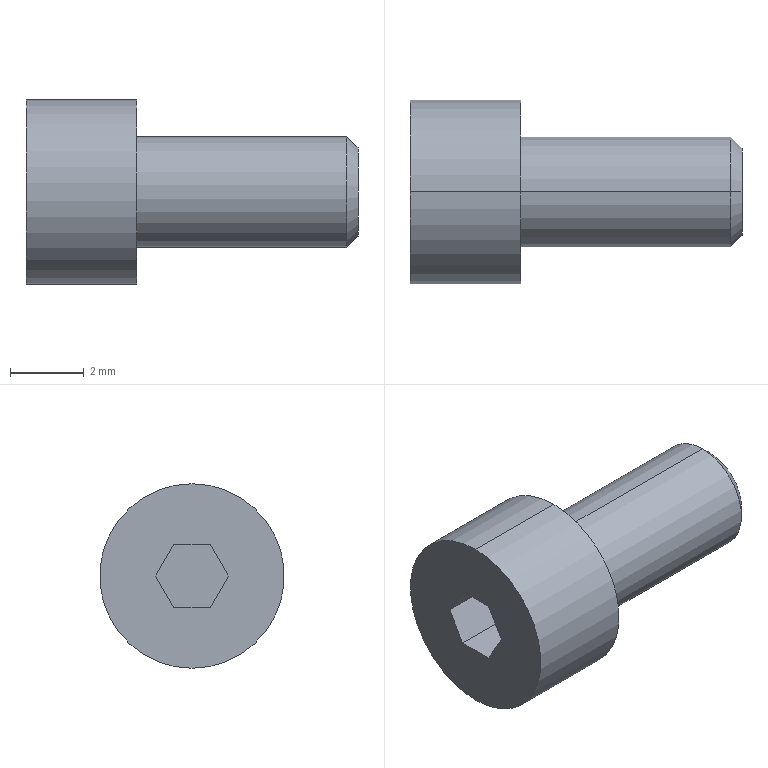Part | SolidWorks | features BaseBody 1 | 1 solid | 16 faces | box 9 x 5 x 5 mm | volume 97.086 mm3 | plane 10 | cylinder 4 | cone 2 | commonest cylinder face diameters 3 x2 5 x2
STEP:
#1=CARTESIAN_POINT('',(9.,0.,1.194));
#2=VERTEX_POINT('',#1);
#3=CARTESIAN_POINT('',(9.,0.,-1.194));
#4=VERTEX_POINT('',#3);
#5=CARTESIAN_POINT('',(9.,0.,0.));
#6=DIRECTION('',(-1.,0.,0.));
#7=DIRECTION('',(0.,0.,1.));
#8=AXIS2_PLACEMENT_3D('',#5,#6,#7);
#9=CIRCLE('',#8,1.194);
#10=EDGE_CURVE('',#2,#4,#9,.T.);
#11=ORIENTED_EDGE('',*,*,#10,.T.);
#12=CARTESIAN_POINT('',(8.694,0.,-1.5));
#13=VERTEX_POINT('',#12);
#14=CARTESIAN_POINT('',(9.,0.,-1.194));
#15=DIRECTION('',(-0.7071,0.,-0.7071));
#16=VECTOR('',#15,1000.);
#17=LINE('',#14,#16);
#18=EDGE_CURVE('',#4,#13,#17,.T.);
#19=ORIENTED_EDGE('',*,*,#18,.T.);
#20=CARTESIAN_POINT('',(8.694,0.,1.5));
#21=VERTEX_POINT('',#20);
#22=CARTESIAN_POINT('',(8.694,0.,0.));
#23=DIRECTION('',(-1.,0.,0.));
#24=DIRECTION('',(0.,0.,1.));
#25=AXIS2_PLACEMENT_3D('',#22,#23,#24);
#26=CIRCLE('',#25,1.5);
#27=EDGE_CURVE('',#21,#13,#26,.T.);
#28=ORIENTED_EDGE('',*,*,#27,.F.);
#29=CARTESIAN_POINT('',(9.,0.,1.194));
#30=DIRECTION('',(-0.7071,0.,0.7071));
#31=VECTOR('',#30,1000.);
#32=LINE('',#29,#31);
#33=EDGE_CURVE('',#2,#21,#32,.T.);
#34=ORIENTED_EDGE('',*,*,#33,.F.);
#35=EDGE_LOOP('',(#11,#19,#28,#34));
#36=FACE_OUTER_BOUND('',#35,.T.);
#37=CARTESIAN_POINT('',(9.,0.,0.));
#38=DIRECTION('',(-1.,0.,0.));
#39=DIRECTION('',(0.,0.,1.));
#40=AXIS2_PLACEMENT_3D('',#37,#38,#39);
#41=CONICAL_SURFACE('',#40,1.194,0.7854);
#42=ADVANCED_FACE('',(#36),#41,.T.);
#43=CARTESIAN_POINT('',(0.,0.,-2.5));
#44=VERTEX_POINT('',#43);
#45=CARTESIAN_POINT('',(0.,0.,2.5));
#46=VERTEX_POINT('',#45);
#47=CARTESIAN_POINT('',(0.,0.,0.));
#48=DIRECTION('',(-1.,0.,0.));
#49=DIRECTION('',(0.,0.,1.));
#50=AXIS2_PLACEMENT_3D('',#47,#48,#49);
#51=CIRCLE('',#50,2.5);
#52=EDGE_CURVE('',#44,#46,#51,.T.);
#53=ORIENTED_EDGE('',*,*,#52,.F.);
#54=CARTESIAN_POINT('',(3.,0.,-2.5));
#55=VERTEX_POINT('',#54);
#56=CARTESIAN_POINT('',(0.,0.,-2.5));
#57=DIRECTION('',(1.,0.,0.));
#58=VECTOR('',#57,1000.);
#59=LINE('',#56,#58);
#60=EDGE_CURVE('',#44,#55,#59,.T.);
#61=ORIENTED_EDGE('',*,*,#60,.T.);
#62=CARTESIAN_POINT('',(3.,0.,2.5));
#63=VERTEX_POINT('',#62);
#64=CARTESIAN_POINT('',(3.,0.,0.));
#65=DIRECTION('',(-1.,0.,0.));
#66=DIRECTION('',(0.,0.,1.));
#67=AXIS2_PLACEMENT_3D('',#64,#65,#66);
#68=CIRCLE('',#67,2.5);
#69=EDGE_CURVE('',#55,#63,#68,.T.);
#70=ORIENTED_EDGE('',*,*,#69,.T.);
#71=CARTESIAN_POINT('',(0.,0.,2.5));
#72=DIRECTION('',(1.,0.,0.));
#73=VECTOR('',#72,1000.);
#74=LINE('',#71,#73);
#75=EDGE_CURVE('',#46,#63,#74,.T.);
#76=ORIENTED_EDGE('',*,*,#75,.F.);
#77=EDGE_LOOP('',(#53,#61,#70,#76));
#78=FACE_OUTER_BOUND('',#77,.T.);
#79=CARTESIAN_POINT('',(0.,0.,0.));
#80=DIRECTION('',(1.,0.,0.));
#81=DIRECTION('',(0.,0.,1.));
#82=AXIS2_PLACEMENT_3D('',#79,#80,#81);
#83=CYLINDRICAL_SURFACE('',#82,2.5);
#84=ADVANCED_FACE('',(#78),#83,.T.);
#85=CARTESIAN_POINT('',(3.,0.,-1.5));
#86=VERTEX_POINT('',#85);
#87=CARTESIAN_POINT('',(3.,0.,1.5));
#88=VERTEX_POINT('',#87);
#89=CARTESIAN_POINT('',(3.,0.,0.));
#90=DIRECTION('',(-1.,0.,0.));
#91=DIRECTION('',(0.,0.,1.));
#92=AXIS2_PLACEMENT_3D('',#89,#90,#91);
#93=CIRCLE('',#92,1.5);
#94=EDGE_CURVE('',#86,#88,#93,.T.);
#95=ORIENTED_EDGE('',*,*,#94,.F.);
#96=CARTESIAN_POINT('',(0.,0.,-1.5));
#97=DIRECTION('',(1.,0.,0.));
#98=VECTOR('',#97,1000.);
#99=LINE('',#96,#98);
#100=EDGE_CURVE('',#86,#13,#99,.T.);
#101=ORIENTED_EDGE('',*,*,#100,.T.);
#102=CARTESIAN_POINT('',(8.694,0.,0.));
#103=DIRECTION('',(-1.,0.,0.));
#104=DIRECTION('',(0.,0.,1.));
#105=AXIS2_PLACEMENT_3D('',#102,#103,#104);
#106=CIRCLE('',#105,1.5);
#107=EDGE_CURVE('',#13,#21,#106,.T.);
#108=ORIENTED_EDGE('',*,*,#107,.T.);
#109=CARTESIAN_POINT('',(0.,0.,1.5));
#110=DIRECTION('',(1.,0.,0.));
#111=VECTOR('',#110,1000.);
#112=LINE('',#109,#111);
#113=EDGE_CURVE('',#88,#21,#112,.T.);
#114=ORIENTED_EDGE('',*,*,#113,.F.);
#115=EDGE_LOOP('',(#95,#101,#108,#114));
#116=FACE_OUTER_BOUND('',#115,.T.);
#117=CARTESIAN_POINT('',(0.,0.,0.));
#118=DIRECTION('',(1.,0.,0.));
#119=DIRECTION('',(0.,0.,1.));
#120=AXIS2_PLACEMENT_3D('',#117,#118,#119);
#121=CYLINDRICAL_SURFACE('',#120,1.5);
#122=ADVANCED_FACE('',(#116),#121,.T.);
#123=CARTESIAN_POINT('',(1.5,0.4949,0.8571));
#124=VERTEX_POINT('',#123);
#125=CARTESIAN_POINT('',(1.5,-0.4949,0.8571));
#126=VERTEX_POINT('',#125);
#127=CARTESIAN_POINT('',(1.5,0.4949,0.8571));
#128=DIRECTION('',(0.,-1.,0.));
#129=VECTOR('',#128,1000.);
#130=LINE('',#127,#129);
#131=EDGE_CURVE('',#124,#126,#130,.T.);
#132=ORIENTED_EDGE('',*,*,#131,.F.);
#133=CARTESIAN_POINT('',(1.5,0.9897,0.));
#134=VERTEX_POINT('',#133);
#135=CARTESIAN_POINT('',(1.5,0.9897,0.));
#136=DIRECTION('',(0.,-0.5,0.866));
#137=VECTOR('',#136,1000.);
#138=LINE('',#135,#137);
#139=EDGE_CURVE('',#134,#124,#138,.T.);
#140=ORIENTED_EDGE('',*,*,#139,.F.);
#141=CARTESIAN_POINT('',(1.5,0.4949,-0.8571));
#142=VERTEX_POINT('',#141);
#143=CARTESIAN_POINT('',(1.5,0.4949,-0.8571));
#144=DIRECTION('',(0.,0.5,0.866));
#145=VECTOR('',#144,1000.);
#146=LINE('',#143,#145);
#147=EDGE_CURVE('',#142,#134,#146,.T.);
#148=ORIENTED_EDGE('',*,*,#147,.F.);
#149=CARTESIAN_POINT('',(1.5,-0.4949,-0.8571));
#150=VERTEX_POINT('',#149);
#151=CARTESIAN_POINT('',(1.5,-0.4949,-0.8571));
#152=DIRECTION('',(0.,1.,0.));
#153=VECTOR('',#152,1000.);
#154=LINE('',#151,#153);
#155=EDGE_CURVE('',#150,#142,#154,.T.);
#156=ORIENTED_EDGE('',*,*,#155,.F.);
#157=CARTESIAN_POINT('',(1.5,-0.9897,0.));
#158=VERTEX_POINT('',#157);
#159=CARTESIAN_POINT('',(1.5,-0.9897,0.));
#160=DIRECTION('',(0.,0.5,-0.866));
#161=VECTOR('',#160,1000.);
#162=LINE('',#159,#161);
#163=EDGE_CURVE('',#158,#150,#162,.T.);
#164=ORIENTED_EDGE('',*,*,#163,.F.);
#165=CARTESIAN_POINT('',(1.5,-0.4949,0.8571));
#166=DIRECTION('',(0.,-0.5,-0.866));
#167=VECTOR('',#166,1000.);
#168=LINE('',#165,#167);
#169=EDGE_CURVE('',#126,#158,#168,.T.);
#170=ORIENTED_EDGE('',*,*,#169,.F.);
#171=EDGE_LOOP('',(#132,#140,#148,#156,#164,#170));
#172=FACE_OUTER_BOUND('',#171,.T.);
#173=CARTESIAN_POINT('',(1.5,0.,0.));
#174=DIRECTION('',(1.,0.,0.));
#175=DIRECTION('',(0.,1.,0.));
#176=AXIS2_PLACEMENT_3D('',#173,#174,#175);
#177=PLANE('',#176);
#178=ADVANCED_FACE('',(#172),#177,.F.);
#179=CARTESIAN_POINT('',(0.,0.9897,0.));
#180=VERTEX_POINT('',#179);
#181=CARTESIAN_POINT('',(0.,0.4949,0.8571));
#182=VERTEX_POINT('',#181);
#183=CARTESIAN_POINT('',(0.,0.9897,0.));
#184=DIRECTION('',(0.,-0.5,0.866));
#185=VECTOR('',#184,1000.);
#186=LINE('',#183,#185);
#187=EDGE_CURVE('',#180,#182,#186,.T.);
#188=ORIENTED_EDGE('',*,*,#187,.F.);
#189=CARTESIAN_POINT('',(1.5,0.9897,0.));
#190=DIRECTION('',(-1.,0.,0.));
#191=VECTOR('',#190,1000.);
#192=LINE('',#189,#191);
#193=EDGE_CURVE('',#134,#180,#192,.T.);
#194=ORIENTED_EDGE('',*,*,#193,.F.);
#195=ORIENTED_EDGE('',*,*,#139,.T.);
#196=CARTESIAN_POINT('',(1.5,0.4949,0.8571));
#197=DIRECTION('',(-1.,0.,0.));
#198=VECTOR('',#197,1000.);
#199=LINE('',#196,#198);
#200=EDGE_CURVE('',#124,#182,#199,.T.);
#201=ORIENTED_EDGE('',*,*,#200,.T.);
#202=EDGE_LOOP('',(#188,#194,#195,#201));
#203=FACE_OUTER_BOUND('',#202,.T.);
#204=CARTESIAN_POINT('',(1.5,0.9897,0.));
#205=DIRECTION('',(0.,-0.866,-0.5));
#206=DIRECTION('',(0.,0.5,-0.866));
#207=AXIS2_PLACEMENT_3D('',#204,#205,#206);
#208=PLANE('',#207);
#209=ADVANCED_FACE('',(#203),#208,.T.);
#210=CARTESIAN_POINT('',(0.,0.4949,-0.8571));
#211=VERTEX_POINT('',#210);
#212=CARTESIAN_POINT('',(0.,0.4949,-0.8571));
#213=DIRECTION('',(0.,0.5,0.866));
#214=VECTOR('',#213,1000.);
#215=LINE('',#212,#214);
#216=EDGE_CURVE('',#211,#180,#215,.T.);
#217=ORIENTED_EDGE('',*,*,#216,.F.);
#218=CARTESIAN_POINT('',(1.5,0.4949,-0.8571));
#219=DIRECTION('',(-1.,0.,0.));
#220=VECTOR('',#219,1000.);
#221=LINE('',#218,#220);
#222=EDGE_CURVE('',#142,#211,#221,.T.);
#223=ORIENTED_EDGE('',*,*,#222,.F.);
#224=ORIENTED_EDGE('',*,*,#147,.T.);
#225=ORIENTED_EDGE('',*,*,#193,.T.);
#226=EDGE_LOOP('',(#217,#223,#224,#225));
#227=FACE_OUTER_BOUND('',#226,.T.);
#228=CARTESIAN_POINT('',(1.5,0.4949,-0.8571));
#229=DIRECTION('',(0.,-0.866,0.5));
#230=DIRECTION('',(-1.,0.,0.));
#231=AXIS2_PLACEMENT_3D('',#228,#229,#230);
#232=PLANE('',#231);
#233=ADVANCED_FACE('',(#227),#232,.T.);
#234=CARTESIAN_POINT('',(0.,-0.4949,-0.8571));
#235=VERTEX_POINT('',#234);
#236=CARTESIAN_POINT('',(0.,-0.4949,-0.8571));
#237=DIRECTION('',(0.,1.,0.));
#238=VECTOR('',#237,1000.);
#239=LINE('',#236,#238);
#240=EDGE_CURVE('',#235,#211,#239,.T.);
#241=ORIENTED_EDGE('',*,*,#240,.F.);
#242=CARTESIAN_POINT('',(1.5,-0.4949,-0.8571));
#243=DIRECTION('',(-1.,0.,0.));
#244=VECTOR('',#243,1000.);
#245=LINE('',#242,#244);
#246=EDGE_CURVE('',#150,#235,#245,.T.);
#247=ORIENTED_EDGE('',*,*,#246,.F.);
#248=ORIENTED_EDGE('',*,*,#155,.T.);
#249=ORIENTED_EDGE('',*,*,#222,.T.);
#250=EDGE_LOOP('',(#241,#247,#248,#249));
#251=FACE_OUTER_BOUND('',#250,.T.);
#252=CARTESIAN_POINT('',(1.5,-0.4949,-0.8571));
#253=DIRECTION('',(0.,0.,1.));
#254=DIRECTION('',(1.,0.,0.));
#255=AXIS2_PLACEMENT_3D('',#252,#253,#254);
#256=PLANE('',#255);
#257=ADVANCED_FACE('',(#251),#256,.T.);
#258=CARTESIAN_POINT('',(0.,-0.9897,0.));
#259=VERTEX_POINT('',#258);
#260=CARTESIAN_POINT('',(0.,-0.9897,0.));
#261=DIRECTION('',(0.,0.5,-0.866));
#262=VECTOR('',#261,1000.);
#263=LINE('',#260,#262);
#264=EDGE_CURVE('',#259,#235,#263,.T.);
#265=ORIENTED_EDGE('',*,*,#264,.F.);
#266=CARTESIAN_POINT('',(1.5,-0.9897,0.));
#267=DIRECTION('',(-1.,0.,0.));
#268=VECTOR('',#267,1000.);
#269=LINE('',#266,#268);
#270=EDGE_CURVE('',#158,#259,#269,.T.);
#271=ORIENTED_EDGE('',*,*,#270,.F.);
#272=ORIENTED_EDGE('',*,*,#163,.T.);
#273=ORIENTED_EDGE('',*,*,#246,.T.);
#274=EDGE_LOOP('',(#265,#271,#272,#273));
#275=FACE_OUTER_BOUND('',#274,.T.);
#276=CARTESIAN_POINT('',(1.5,-0.9897,0.));
#277=DIRECTION('',(0.,0.866,0.5));
#278=DIRECTION('',(1.,0.,0.));
#279=AXIS2_PLACEMENT_3D('',#276,#277,#278);
#280=PLANE('',#279);
#281=ADVANCED_FACE('',(#275),#280,.T.);
#282=CARTESIAN_POINT('',(0.,-0.4949,0.8571));
#283=VERTEX_POINT('',#282);
#284=CARTESIAN_POINT('',(0.,-0.4949,0.8571));
#285=DIRECTION('',(0.,-0.5,-0.866));
#286=VECTOR('',#285,1000.);
#287=LINE('',#284,#286);
#288=EDGE_CURVE('',#283,#259,#287,.T.);
#289=ORIENTED_EDGE('',*,*,#288,.F.);
#290=CARTESIAN_POINT('',(1.5,-0.4949,0.8571));
#291=DIRECTION('',(-1.,0.,0.));
#292=VECTOR('',#291,1000.);
#293=LINE('',#290,#292);
#294=EDGE_CURVE('',#126,#283,#293,.T.);
#295=ORIENTED_EDGE('',*,*,#294,.F.);
#296=ORIENTED_EDGE('',*,*,#169,.T.);
#297=ORIENTED_EDGE('',*,*,#270,.T.);
#298=EDGE_LOOP('',(#289,#295,#296,#297));
#299=FACE_OUTER_BOUND('',#298,.T.);
#300=CARTESIAN_POINT('',(1.5,-0.4949,0.8571));
#301=DIRECTION('',(0.,0.866,-0.5));
#302=DIRECTION('',(-1.,0.,0.));
#303=AXIS2_PLACEMENT_3D('',#300,#301,#302);
#304=PLANE('',#303);
#305=ADVANCED_FACE('',(#299),#304,.T.);
#306=CARTESIAN_POINT('',(0.,0.4949,0.8571));
#307=DIRECTION('',(0.,-1.,0.));
#308=VECTOR('',#307,1000.);
#309=LINE('',#306,#308);
#310=EDGE_CURVE('',#182,#283,#309,.T.);
#311=ORIENTED_EDGE('',*,*,#310,.F.);
#312=ORIENTED_EDGE('',*,*,#200,.F.);
#313=ORIENTED_EDGE('',*,*,#131,.T.);
#314=ORIENTED_EDGE('',*,*,#294,.T.);
#315=EDGE_LOOP('',(#311,#312,#313,#314));
#316=FACE_OUTER_BOUND('',#315,.T.);
#317=CARTESIAN_POINT('',(1.5,0.4949,0.8571));
#318=DIRECTION('',(0.,0.,-1.));
#319=DIRECTION('',(0.,-1.,0.));
#320=AXIS2_PLACEMENT_3D('',#317,#318,#319);
#321=PLANE('',#320);
#322=ADVANCED_FACE('',(#316),#321,.T.);
#323=ORIENTED_EDGE('',*,*,#100,.F.);
#324=CARTESIAN_POINT('',(3.,0.,0.));
#325=DIRECTION('',(-1.,0.,0.));
#326=DIRECTION('',(0.,0.,1.));
#327=AXIS2_PLACEMENT_3D('',#324,#325,#326);
#328=CIRCLE('',#327,1.5);
#329=EDGE_CURVE('',#88,#86,#328,.T.);
#330=ORIENTED_EDGE('',*,*,#329,.F.);
#331=ORIENTED_EDGE('',*,*,#113,.T.);
#332=ORIENTED_EDGE('',*,*,#27,.T.);
#333=EDGE_LOOP('',(#323,#330,#331,#332));
#334=FACE_OUTER_BOUND('',#333,.T.);
#335=CARTESIAN_POINT('',(0.,0.,0.));
#336=DIRECTION('',(1.,0.,0.));
#337=DIRECTION('',(0.,0.,1.));
#338=AXIS2_PLACEMENT_3D('',#335,#336,#337);
#339=CYLINDRICAL_SURFACE('',#338,1.5);
#340=ADVANCED_FACE('',(#334),#339,.T.);
#341=ORIENTED_EDGE('',*,*,#329,.T.);
#342=ORIENTED_EDGE('',*,*,#94,.T.);
#343=EDGE_LOOP('',(#341,#342));
#344=FACE_BOUND('',#343,.T.);
#345=CARTESIAN_POINT('',(3.,0.,0.));
#346=DIRECTION('',(-1.,0.,0.));
#347=DIRECTION('',(0.,0.,1.));
#348=AXIS2_PLACEMENT_3D('',#345,#346,#347);
#349=CIRCLE('',#348,2.5);
#350=EDGE_CURVE('',#63,#55,#349,.T.);
#351=ORIENTED_EDGE('',*,*,#350,.F.);
#352=ORIENTED_EDGE('',*,*,#69,.F.);
#353=EDGE_LOOP('',(#351,#352));
#354=FACE_OUTER_BOUND('',#353,.T.);
#355=CARTESIAN_POINT('',(3.,-1.5,0.));
#356=DIRECTION('',(-1.,0.,0.));
#357=DIRECTION('',(0.,0.,1.));
#358=AXIS2_PLACEMENT_3D('',#355,#356,#357);
#359=PLANE('',#358);
#360=ADVANCED_FACE('',(#344,#354),#359,.F.);
#361=ORIENTED_EDGE('',*,*,#60,.F.);
#362=CARTESIAN_POINT('',(0.,0.,0.));
#363=DIRECTION('',(-1.,0.,0.));
#364=DIRECTION('',(0.,0.,1.));
#365=AXIS2_PLACEMENT_3D('',#362,#363,#364);
#366=CIRCLE('',#365,2.5);
#367=EDGE_CURVE('',#46,#44,#366,.T.);
#368=ORIENTED_EDGE('',*,*,#367,.F.);
#369=ORIENTED_EDGE('',*,*,#75,.T.);
#370=ORIENTED_EDGE('',*,*,#350,.T.);
#371=EDGE_LOOP('',(#361,#368,#369,#370));
#372=FACE_OUTER_BOUND('',#371,.T.);
#373=CARTESIAN_POINT('',(0.,0.,0.));
#374=DIRECTION('',(1.,0.,0.));
#375=DIRECTION('',(0.,0.,1.));
#376=AXIS2_PLACEMENT_3D('',#373,#374,#375);
#377=CYLINDRICAL_SURFACE('',#376,2.5);
#378=ADVANCED_FACE('',(#372),#377,.T.);
#379=ORIENTED_EDGE('',*,*,#288,.T.);
#380=ORIENTED_EDGE('',*,*,#264,.T.);
#381=ORIENTED_EDGE('',*,*,#240,.T.);
#382=ORIENTED_EDGE('',*,*,#216,.T.);
#383=ORIENTED_EDGE('',*,*,#187,.T.);
#384=ORIENTED_EDGE('',*,*,#310,.T.);
#385=EDGE_LOOP('',(#379,#380,#381,#382,#383,#384));
#386=FACE_BOUND('',#385,.T.);
#387=ORIENTED_EDGE('',*,*,#367,.T.);
#388=ORIENTED_EDGE('',*,*,#52,.T.);
#389=EDGE_LOOP('',(#387,#388));
#390=FACE_OUTER_BOUND('',#389,.T.);
#391=CARTESIAN_POINT('',(0.,-2.5,0.));
#392=DIRECTION('',(1.,0.,0.));
#393=DIRECTION('',(0.,1.,0.));
#394=AXIS2_PLACEMENT_3D('',#391,#392,#393);
#395=PLANE('',#394);
#396=ADVANCED_FACE('',(#386,#390),#395,.F.);
#397=ORIENTED_EDGE('',*,*,#10,.F.);
#398=CARTESIAN_POINT('',(9.,0.,0.));
#399=DIRECTION('',(-1.,0.,0.));
#400=DIRECTION('',(0.,0.,1.));
#401=AXIS2_PLACEMENT_3D('',#398,#399,#400);
#402=CIRCLE('',#401,1.194);
#403=EDGE_CURVE('',#4,#2,#402,.T.);
#404=ORIENTED_EDGE('',*,*,#403,.F.);
#405=EDGE_LOOP('',(#397,#404));
#406=FACE_OUTER_BOUND('',#405,.T.);
#407=CARTESIAN_POINT('',(9.,0.,0.));
#408=DIRECTION('',(-1.,0.,0.));
#409=DIRECTION('',(0.,0.,1.));
#410=AXIS2_PLACEMENT_3D('',#407,#408,#409);
#411=PLANE('',#410);
#412=ADVANCED_FACE('',(#406),#411,.F.);
#413=ORIENTED_EDGE('',*,*,#18,.F.);
#414=ORIENTED_EDGE('',*,*,#403,.T.);
#415=ORIENTED_EDGE('',*,*,#33,.T.);
#416=ORIENTED_EDGE('',*,*,#107,.F.);
#417=EDGE_LOOP('',(#413,#414,#415,#416));
#418=FACE_OUTER_BOUND('',#417,.T.);
#419=CARTESIAN_POINT('',(9.,0.,0.));
#420=DIRECTION('',(-1.,0.,0.));
#421=DIRECTION('',(0.,0.,1.));
#422=AXIS2_PLACEMENT_3D('',#419,#420,#421);
#423=CONICAL_SURFACE('',#422,1.194,0.7854);
#424=ADVANCED_FACE('',(#418),#423,.T.);
#425=CLOSED_SHELL('',(#42,#84,#122,#178,#209,#233,#257,#281,#305,#322,#340,#360,#378,#396,#412,#424));
#426=MANIFOLD_SOLID_BREP('',#425);
#427=CARTESIAN_POINT('',(0.,0.,0.));
#428=DIRECTION('',(0.,0.,1.));
#429=DIRECTION('',(1.,0.,0.));
#430=AXIS2_PLACEMENT_3D('',#427,#428,#429);
#431=(LENGTH_UNIT()NAMED_UNIT(*)SI_UNIT(.MILLI.,.METRE.));
#432=UNCERTAINTY_MEASURE_WITH_UNIT(LENGTH_MEASURE(0.00001),#431,'','');
#433=(NAMED_UNIT(*)PLANE_ANGLE_UNIT()SI_UNIT($,.RADIAN.));
#434=(NAMED_UNIT(*)SI_UNIT($,.STERADIAN.)SOLID_ANGLE_UNIT());
#435=(GEOMETRIC_REPRESENTATION_CONTEXT(3)GLOBAL_UNCERTAINTY_ASSIGNED_CONTEXT((#432))GLOBAL_UNIT_ASSIGNED_CONTEXT((#431,#433,#434))REPRESENTATION_CONTEXT('',''));
#436=ADVANCED_BREP_SHAPE_REPRESENTATION('',(#426,#430),#435);